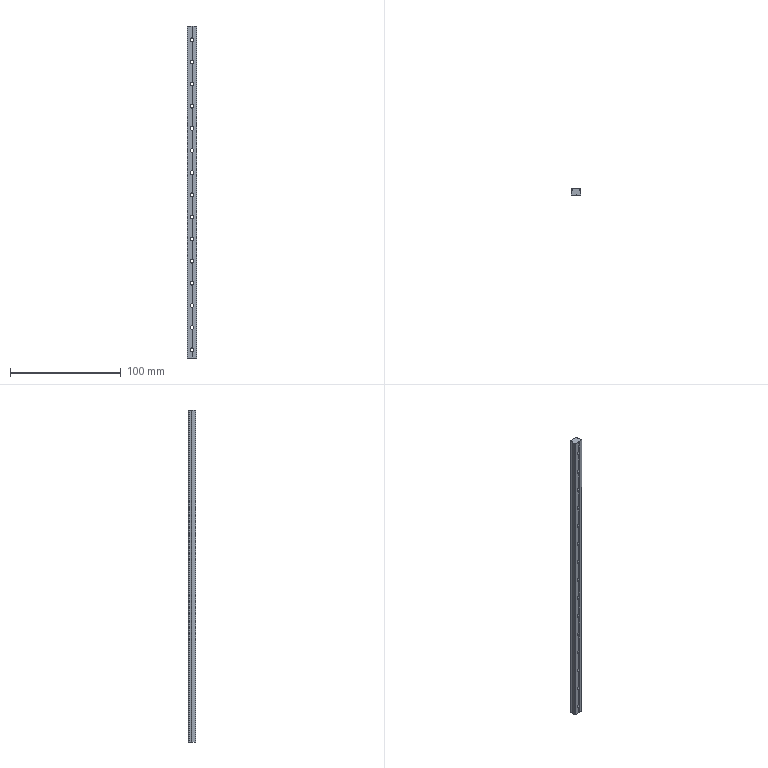Part | STEP file | MANIFOLD_SOLID_BREP_106V1.201001 | 1 solid | 107 faces | box 9 x 6.5 x 300 mm | volume 14670 mm3 | cylinder 79 | plane 28 | commonest cylinder face diameters 6 x30 3.4 x22 0.6 x16 3.5 x8 2 x3